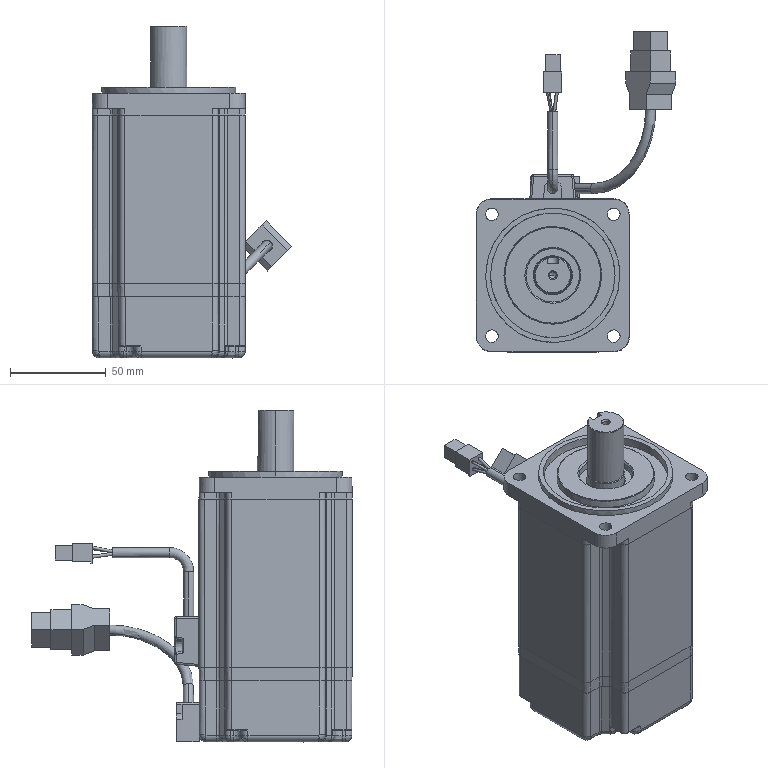Part | SolidWorks | features BaseBody 1 | 1 solid | 2066 faces | box 104.241 x 167.272 x 173.3 mm | volume 816769 mm3 | plane 1271 | spline 522 | cylinder 184 | cone 33 | torus 28 | sphere 28 | commonest cylinder face diameters 7 x30 6 x29 4 x24 2 x20 0.6 x8 1.5 x8